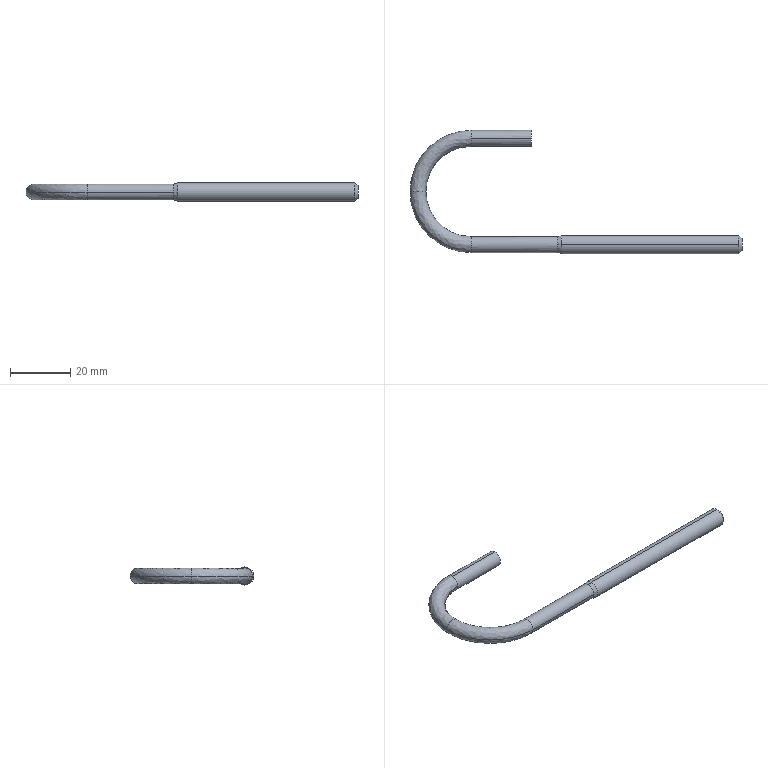Part | STEP file | 750038353 | 1 solid | 16 faces | box 110.3 x 40.95 x 6 mm | volume 4017 mm3 | spline 6 | cylinder 6 | cone 2 | plane 2 | commonest cylinder face diameters 5.3 x4 6 x2
STEP:
#1=CARTESIAN_POINT('',(28.594,-17.65,2.65));
#2=VERTEX_POINT('',#1);
#3=CARTESIAN_POINT('',(28.594,-15.,0.));
#4=VERTEX_POINT('',#3);
#5=CARTESIAN_POINT('',(28.594,-17.65,0.));
#6=DIRECTION('',(-1.,0.,0.));
#7=DIRECTION('',(0.,0.,-1.));
#8=AXIS2_PLACEMENT_3D('',#5,#6,#7);
#9=CIRCLE('',#8,2.65);
#10=EDGE_CURVE('',#2,#4,#9,.T.);
#11=ORIENTED_EDGE('',*,*,#10,.F.);
#12=CARTESIAN_POINT('',(30.,-17.65,3.));
#13=VERTEX_POINT('',#12);
#14=CARTESIAN_POINT('',(28.594,-17.65,5.65));
#15=DIRECTION('',(0.,-1.,0.));
#16=DIRECTION('',(0.,0.,1.));
#17=AXIS2_PLACEMENT_3D('',#14,#15,#16);
#18=CIRCLE('',#17,3.);
#19=EDGE_CURVE('',#2,#13,#18,.T.);
#20=ORIENTED_EDGE('',*,*,#19,.T.);
#21=CARTESIAN_POINT('',(30.,-17.65,-3.));
#22=VERTEX_POINT('',#21);
#23=CARTESIAN_POINT('',(30.,-17.65,0.));
#24=DIRECTION('',(1.,0.,0.));
#25=DIRECTION('',(0.,0.,-1.));
#26=AXIS2_PLACEMENT_3D('',#23,#24,#25);
#27=CIRCLE('',#26,3.);
#28=EDGE_CURVE('',#22,#13,#27,.T.);
#29=ORIENTED_EDGE('',*,*,#28,.F.);
#30=CARTESIAN_POINT('',(28.594,-17.65,-2.65));
#31=VERTEX_POINT('',#30);
#32=CARTESIAN_POINT('',(28.594,-17.65,-5.65));
#33=DIRECTION('',(0.,1.,0.));
#34=DIRECTION('',(0.,0.,-1.));
#35=AXIS2_PLACEMENT_3D('',#32,#33,#34);
#36=CIRCLE('',#35,3.);
#37=EDGE_CURVE('',#31,#22,#36,.T.);
#38=ORIENTED_EDGE('',*,*,#37,.F.);
#39=CARTESIAN_POINT('',(28.594,-17.65,0.));
#40=DIRECTION('',(-1.,0.,0.));
#41=DIRECTION('',(0.,0.,-1.));
#42=AXIS2_PLACEMENT_3D('',#39,#40,#41);
#43=CIRCLE('',#42,2.65);
#44=EDGE_CURVE('',#4,#31,#43,.T.);
#45=ORIENTED_EDGE('',*,*,#44,.F.);
#46=EDGE_LOOP('',(#11,#20,#29,#38,#45));
#47=FACE_OUTER_BOUND('',#46,.T.);
#48=CARTESIAN_POINT('',(28.594,-17.65,-2.65));
#49=CARTESIAN_POINT('',(28.594,-12.35,-2.65));
#50=CARTESIAN_POINT('',(28.594,-12.35,2.65));
#51=CARTESIAN_POINT('',(28.594,-17.65,2.65));
#52=CARTESIAN_POINT('',(29.087,-17.65,-2.65));
#53=CARTESIAN_POINT('',(29.087,-12.35,-2.65));
#54=CARTESIAN_POINT('',(29.087,-12.35,2.65));
#55=CARTESIAN_POINT('',(29.087,-17.65,2.65));
#56=CARTESIAN_POINT('',(29.565,-17.65,-2.769));
#57=CARTESIAN_POINT('',(29.565,-12.112,-2.769));
#58=CARTESIAN_POINT('',(29.565,-12.112,2.769));
#59=CARTESIAN_POINT('',(29.565,-17.65,2.769));
#60=CARTESIAN_POINT('',(30.,-17.65,-3.));
#61=CARTESIAN_POINT('',(30.,-11.65,-3.));
#62=CARTESIAN_POINT('',(30.,-11.65,3.));
#63=CARTESIAN_POINT('',(30.,-17.65,3.));
#64=(BOUNDED_SURFACE()B_SPLINE_SURFACE(3,3,((#48,#49,#50,#51),(#52,#53,#54,#55),(#56,#57,#58,#59),(#60,#61,#62,#63)),.UNSPECIFIED.,.F.,.F.,.F.)B_SPLINE_SURFACE_WITH_KNOTS((4,4),(4,4),(0.,1.),(0.,1.),.UNSPECIFIED.)GEOMETRIC_REPRESENTATION_ITEM()RATIONAL_B_SPLINE_SURFACE(((1.,0.3333,0.3333,1.),(0.9803,0.3268,0.3268,0.9803),(0.9803,0.3268,0.3268,0.9803),(1.,0.3333,0.3333,1.)))REPRESENTATION_ITEM('')SURFACE());
#65=ADVANCED_FACE('',(#47),#64,.F.);
#66=CARTESIAN_POINT('',(-15.,0.,0.));
#67=VERTEX_POINT('',#66);
#68=CARTESIAN_POINT('',(0.,15.,0.));
#69=VERTEX_POINT('',#68);
#70=CARTESIAN_POINT('',(0.,0.,0.));
#71=DIRECTION('',(0.,0.,-1.));
#72=DIRECTION('',(-1.,0.,0.));
#73=AXIS2_PLACEMENT_3D('',#70,#71,#72);
#74=CIRCLE('',#73,15.);
#75=EDGE_CURVE('',#67,#69,#74,.T.);
#76=ORIENTED_EDGE('',*,*,#75,.F.);
#77=CARTESIAN_POINT('',(-20.3,0.,0.));
#78=VERTEX_POINT('',#77);
#79=CARTESIAN_POINT('',(-17.65,0.,0.));
#80=DIRECTION('',(0.,1.,0.));
#81=DIRECTION('',(-1.,0.,0.));
#82=AXIS2_PLACEMENT_3D('',#79,#80,#81);
#83=CIRCLE('',#82,2.65);
#84=EDGE_CURVE('',#67,#78,#83,.T.);
#85=ORIENTED_EDGE('',*,*,#84,.T.);
#86=CARTESIAN_POINT('',(0.,20.3,0.));
#87=VERTEX_POINT('',#86);
#88=CARTESIAN_POINT('',(0.,0.,0.));
#89=DIRECTION('',(0.,0.,-1.));
#90=DIRECTION('',(-1.,0.,0.));
#91=AXIS2_PLACEMENT_3D('',#88,#89,#90);
#92=CIRCLE('',#91,20.3);
#93=EDGE_CURVE('',#78,#87,#92,.T.);
#94=ORIENTED_EDGE('',*,*,#93,.T.);
#95=CARTESIAN_POINT('',(0.,17.65,-2.65));
#96=VERTEX_POINT('',#95);
#97=CARTESIAN_POINT('',(0.,17.65,0.));
#98=DIRECTION('',(-1.,0.,0.));
#99=DIRECTION('',(0.,1.,0.));
#100=AXIS2_PLACEMENT_3D('',#97,#98,#99);
#101=CIRCLE('',#100,2.65);
#102=EDGE_CURVE('',#87,#96,#101,.T.);
#103=ORIENTED_EDGE('',*,*,#102,.T.);
#104=CARTESIAN_POINT('',(0.,17.65,0.));
#105=DIRECTION('',(-1.,0.,0.));
#106=DIRECTION('',(0.,1.,0.));
#107=AXIS2_PLACEMENT_3D('',#104,#105,#106);
#108=CIRCLE('',#107,2.65);
#109=EDGE_CURVE('',#96,#69,#108,.T.);
#110=ORIENTED_EDGE('',*,*,#109,.T.);
#111=EDGE_LOOP('',(#76,#85,#94,#103,#110));
#112=FACE_OUTER_BOUND('',#111,.T.);
#113=CARTESIAN_POINT('',(-15.,0.,0.));
#114=CARTESIAN_POINT('',(-15.,8.787,0.));
#115=CARTESIAN_POINT('',(-8.787,15.,0.));
#116=CARTESIAN_POINT('',(0.,15.,0.));
#117=CARTESIAN_POINT('',(-15.,0.,-5.3));
#118=CARTESIAN_POINT('',(-15.,8.787,-5.3));
#119=CARTESIAN_POINT('',(-8.787,15.,-5.3));
#120=CARTESIAN_POINT('',(0.,15.,-5.3));
#121=CARTESIAN_POINT('',(-20.3,0.,-5.3));
#122=CARTESIAN_POINT('',(-20.3,11.891,-5.3));
#123=CARTESIAN_POINT('',(-11.891,20.3,-5.3));
#124=CARTESIAN_POINT('',(0.,20.3,-5.3));
#125=CARTESIAN_POINT('',(-20.3,0.,0.));
#126=CARTESIAN_POINT('',(-20.3,11.891,0.));
#127=CARTESIAN_POINT('',(-11.891,20.3,0.));
#128=CARTESIAN_POINT('',(0.,20.3,0.));
#129=(BOUNDED_SURFACE()B_SPLINE_SURFACE(3,3,((#113,#114,#115,#116),(#117,#118,#119,#120),(#121,#122,#123,#124),(#125,#126,#127,#128)),.UNSPECIFIED.,.F.,.F.,.F.)B_SPLINE_SURFACE_WITH_KNOTS((4,4),(4,4),(0.,1.),(0.,1.),.UNSPECIFIED.)GEOMETRIC_REPRESENTATION_ITEM()RATIONAL_B_SPLINE_SURFACE(((1.,0.8047,0.8047,1.),(0.3333,0.2682,0.2682,0.3333),(0.3333,0.2682,0.2682,0.3333),(1.,0.8047,0.8047,1.)))REPRESENTATION_ITEM('')SURFACE());
#130=ADVANCED_FACE('',(#112),#129,.T.);
#131=ORIENTED_EDGE('',*,*,#93,.F.);
#132=CARTESIAN_POINT('',(-17.65,0.,0.));
#133=DIRECTION('',(0.,1.,0.));
#134=DIRECTION('',(-1.,0.,0.));
#135=AXIS2_PLACEMENT_3D('',#132,#133,#134);
#136=CIRCLE('',#135,2.65);
#137=EDGE_CURVE('',#78,#67,#136,.T.);
#138=ORIENTED_EDGE('',*,*,#137,.T.);
#139=ORIENTED_EDGE('',*,*,#75,.T.);
#140=CARTESIAN_POINT('',(0.,17.65,2.65));
#141=VERTEX_POINT('',#140);
#142=CARTESIAN_POINT('',(0.,17.65,0.));
#143=DIRECTION('',(-1.,0.,0.));
#144=DIRECTION('',(0.,1.,0.));
#145=AXIS2_PLACEMENT_3D('',#142,#143,#144);
#146=CIRCLE('',#145,2.65);
#147=EDGE_CURVE('',#69,#141,#146,.T.);
#148=ORIENTED_EDGE('',*,*,#147,.T.);
#149=CARTESIAN_POINT('',(0.,17.65,0.));
#150=DIRECTION('',(-1.,0.,0.));
#151=DIRECTION('',(0.,1.,0.));
#152=AXIS2_PLACEMENT_3D('',#149,#150,#151);
#153=CIRCLE('',#152,2.65);
#154=EDGE_CURVE('',#141,#87,#153,.T.);
#155=ORIENTED_EDGE('',*,*,#154,.T.);
#156=EDGE_LOOP('',(#131,#138,#139,#148,#155));
#157=FACE_OUTER_BOUND('',#156,.T.);
#158=CARTESIAN_POINT('',(-20.3,0.,0.));
#159=CARTESIAN_POINT('',(-20.3,11.891,0.));
#160=CARTESIAN_POINT('',(-11.891,20.3,0.));
#161=CARTESIAN_POINT('',(0.,20.3,0.));
#162=CARTESIAN_POINT('',(-20.3,0.,5.3));
#163=CARTESIAN_POINT('',(-20.3,11.891,5.3));
#164=CARTESIAN_POINT('',(-11.891,20.3,5.3));
#165=CARTESIAN_POINT('',(0.,20.3,5.3));
#166=CARTESIAN_POINT('',(-15.,0.,5.3));
#167=CARTESIAN_POINT('',(-15.,8.787,5.3));
#168=CARTESIAN_POINT('',(-8.787,15.,5.3));
#169=CARTESIAN_POINT('',(0.,15.,5.3));
#170=CARTESIAN_POINT('',(-15.,0.,0.));
#171=CARTESIAN_POINT('',(-15.,8.787,0.));
#172=CARTESIAN_POINT('',(-8.787,15.,0.));
#173=CARTESIAN_POINT('',(0.,15.,0.));
#174=(BOUNDED_SURFACE()B_SPLINE_SURFACE(3,3,((#158,#159,#160,#161),(#162,#163,#164,#165),(#166,#167,#168,#169),(#170,#171,#172,#173)),.UNSPECIFIED.,.F.,.F.,.F.)B_SPLINE_SURFACE_WITH_KNOTS((4,4),(4,4),(0.,1.),(0.,1.),.UNSPECIFIED.)GEOMETRIC_REPRESENTATION_ITEM()RATIONAL_B_SPLINE_SURFACE(((1.,0.8047,0.8047,1.),(0.3333,0.2682,0.2682,0.3333),(0.3333,0.2682,0.2682,0.3333),(1.,0.8047,0.8047,1.)))REPRESENTATION_ITEM('')SURFACE());
#175=ADVANCED_FACE('',(#157),#174,.T.);
#176=ORIENTED_EDGE('',*,*,#28,.T.);
#177=CARTESIAN_POINT('',(89.,-17.65,3.));
#178=VERTEX_POINT('',#177);
#179=CARTESIAN_POINT('',(30.,-17.65,3.));
#180=DIRECTION('',(1.,0.,0.));
#181=VECTOR('',#180,1000.);
#182=LINE('',#179,#181);
#183=EDGE_CURVE('',#13,#178,#182,.T.);
#184=ORIENTED_EDGE('',*,*,#183,.T.);
#185=CARTESIAN_POINT('',(89.,-17.65,-3.));
#186=VERTEX_POINT('',#185);
#187=CARTESIAN_POINT('',(89.,-17.65,0.));
#188=DIRECTION('',(-1.,0.,0.));
#189=DIRECTION('',(0.,0.,-1.));
#190=AXIS2_PLACEMENT_3D('',#187,#188,#189);
#191=CIRCLE('',#190,3.);
#192=EDGE_CURVE('',#178,#186,#191,.T.);
#193=ORIENTED_EDGE('',*,*,#192,.T.);
#194=CARTESIAN_POINT('',(30.,-17.65,-3.));
#195=DIRECTION('',(1.,0.,0.));
#196=VECTOR('',#195,1000.);
#197=LINE('',#194,#196);
#198=EDGE_CURVE('',#22,#186,#197,.T.);
#199=ORIENTED_EDGE('',*,*,#198,.F.);
#200=EDGE_LOOP('',(#176,#184,#193,#199));
#201=FACE_OUTER_BOUND('',#200,.T.);
#202=CARTESIAN_POINT('',(30.,-17.65,0.));
#203=DIRECTION('',(1.,0.,0.));
#204=DIRECTION('',(0.,0.,-1.));
#205=AXIS2_PLACEMENT_3D('',#202,#203,#204);
#206=CYLINDRICAL_SURFACE('',#205,3.);
#207=ADVANCED_FACE('',(#201),#206,.T.);
#208=CARTESIAN_POINT('',(90.,-17.65,2.));
#209=VERTEX_POINT('',#208);
#210=CARTESIAN_POINT('',(90.,-17.65,-2.));
#211=VERTEX_POINT('',#210);
#212=CARTESIAN_POINT('',(90.,-17.65,0.));
#213=DIRECTION('',(-1.,0.,0.));
#214=DIRECTION('',(0.,0.,1.));
#215=AXIS2_PLACEMENT_3D('',#212,#213,#214);
#216=CIRCLE('',#215,2.);
#217=EDGE_CURVE('',#209,#211,#216,.T.);
#218=ORIENTED_EDGE('',*,*,#217,.T.);
#219=CARTESIAN_POINT('',(89.,-17.65,-3.));
#220=DIRECTION('',(-0.7071,0.,-0.7071));
#221=VECTOR('',#220,1000.);
#222=LINE('',#219,#221);
#223=EDGE_CURVE('',#211,#186,#222,.T.);
#224=ORIENTED_EDGE('',*,*,#223,.T.);
#225=ORIENTED_EDGE('',*,*,#192,.F.);
#226=CARTESIAN_POINT('',(89.,-17.65,3.));
#227=DIRECTION('',(-0.7071,0.,0.7071));
#228=VECTOR('',#227,1000.);
#229=LINE('',#226,#228);
#230=EDGE_CURVE('',#209,#178,#229,.T.);
#231=ORIENTED_EDGE('',*,*,#230,.F.);
#232=EDGE_LOOP('',(#218,#224,#225,#231));
#233=FACE_OUTER_BOUND('',#232,.T.);
#234=CARTESIAN_POINT('',(89.,-17.65,0.));
#235=DIRECTION('',(-1.,0.,0.));
#236=DIRECTION('',(0.,0.,1.));
#237=AXIS2_PLACEMENT_3D('',#234,#235,#236);
#238=CONICAL_SURFACE('',#237,3.,0.7854);
#239=ADVANCED_FACE('',(#233),#238,.T.);
#240=CARTESIAN_POINT('',(0.,-15.,0.));
#241=VERTEX_POINT('',#240);
#242=CARTESIAN_POINT('',(0.,-20.3,0.));
#243=VERTEX_POINT('',#242);
#244=CARTESIAN_POINT('',(0.,-17.65,0.));
#245=DIRECTION('',(1.,0.,0.));
#246=DIRECTION('',(0.,1.,0.));
#247=AXIS2_PLACEMENT_3D('',#244,#245,#246);
#248=CIRCLE('',#247,2.65);
#249=EDGE_CURVE('',#241,#243,#248,.T.);
#250=ORIENTED_EDGE('',*,*,#249,.T.);
#251=CARTESIAN_POINT('',(28.594,-20.3,0.));
#252=VERTEX_POINT('',#251);
#253=CARTESIAN_POINT('',(0.,-20.3,0.));
#254=DIRECTION('',(1.,0.,0.));
#255=VECTOR('',#254,1000.);
#256=LINE('',#253,#255);
#257=EDGE_CURVE('',#243,#252,#256,.T.);
#258=ORIENTED_EDGE('',*,*,#257,.T.);
#259=CARTESIAN_POINT('',(28.594,-17.65,0.));
#260=DIRECTION('',(-1.,0.,0.));
#261=DIRECTION('',(0.,0.,-1.));
#262=AXIS2_PLACEMENT_3D('',#259,#260,#261);
#263=CIRCLE('',#262,2.65);
#264=EDGE_CURVE('',#252,#2,#263,.T.);
#265=ORIENTED_EDGE('',*,*,#264,.T.);
#266=ORIENTED_EDGE('',*,*,#10,.T.);
#267=CARTESIAN_POINT('',(0.,-15.,0.));
#268=DIRECTION('',(1.,0.,0.));
#269=VECTOR('',#268,1000.);
#270=LINE('',#267,#269);
#271=EDGE_CURVE('',#241,#4,#270,.T.);
#272=ORIENTED_EDGE('',*,*,#271,.F.);
#273=EDGE_LOOP('',(#250,#258,#265,#266,#272));
#274=FACE_OUTER_BOUND('',#273,.T.);
#275=CARTESIAN_POINT('',(0.,-17.65,0.));
#276=DIRECTION('',(1.,0.,0.));
#277=DIRECTION('',(0.,1.,0.));
#278=AXIS2_PLACEMENT_3D('',#275,#276,#277);
#279=CYLINDRICAL_SURFACE('',#278,2.65);
#280=ADVANCED_FACE('',(#274),#279,.T.);
#281=ORIENTED_EDGE('',*,*,#137,.F.);
#282=CARTESIAN_POINT('',(0.,0.,0.));
#283=DIRECTION('',(0.,0.,-1.));
#284=DIRECTION('',(-1.,0.,0.));
#285=AXIS2_PLACEMENT_3D('',#282,#283,#284);
#286=CIRCLE('',#285,20.3);
#287=EDGE_CURVE('',#243,#78,#286,.T.);
#288=ORIENTED_EDGE('',*,*,#287,.F.);
#289=ORIENTED_EDGE('',*,*,#249,.F.);
#290=CARTESIAN_POINT('',(0.,0.,0.));
#291=DIRECTION('',(0.,0.,-1.));
#292=DIRECTION('',(-1.,0.,0.));
#293=AXIS2_PLACEMENT_3D('',#290,#291,#292);
#294=CIRCLE('',#293,15.);
#295=EDGE_CURVE('',#241,#67,#294,.T.);
#296=ORIENTED_EDGE('',*,*,#295,.T.);
#297=EDGE_LOOP('',(#281,#288,#289,#296));
#298=FACE_OUTER_BOUND('',#297,.T.);
#299=CARTESIAN_POINT('',(0.,-20.3,0.));
#300=CARTESIAN_POINT('',(-11.891,-20.3,0.));
#301=CARTESIAN_POINT('',(-20.3,-11.891,0.));
#302=CARTESIAN_POINT('',(-20.3,0.,0.));
#303=CARTESIAN_POINT('',(0.,-20.3,5.3));
#304=CARTESIAN_POINT('',(-11.891,-20.3,5.3));
#305=CARTESIAN_POINT('',(-20.3,-11.891,5.3));
#306=CARTESIAN_POINT('',(-20.3,0.,5.3));
#307=CARTESIAN_POINT('',(0.,-15.,5.3));
#308=CARTESIAN_POINT('',(-8.787,-15.,5.3));
#309=CARTESIAN_POINT('',(-15.,-8.787,5.3));
#310=CARTESIAN_POINT('',(-15.,0.,5.3));
#311=CARTESIAN_POINT('',(0.,-15.,0.));
#312=CARTESIAN_POINT('',(-8.787,-15.,0.));
#313=CARTESIAN_POINT('',(-15.,-8.787,0.));
#314=CARTESIAN_POINT('',(-15.,0.,0.));
#315=(BOUNDED_SURFACE()B_SPLINE_SURFACE(3,3,((#299,#300,#301,#302),(#303,#304,#305,#306),(#307,#308,#309,#310),(#311,#312,#313,#314)),.UNSPECIFIED.,.F.,.F.,.T.)B_SPLINE_SURFACE_WITH_KNOTS((4,4),(4,4),(0.,1.),(0.,1.),.UNSPECIFIED.)GEOMETRIC_REPRESENTATION_ITEM()RATIONAL_B_SPLINE_SURFACE(((1.,0.8047,0.8047,1.),(0.3333,0.2682,0.2682,0.3333),(0.3333,0.2682,0.2682,0.3333),(1.,0.8047,0.8047,1.)))REPRESENTATION_ITEM('')SURFACE());
#316=ADVANCED_FACE('',(#298),#315,.T.);
#317=ORIENTED_EDGE('',*,*,#154,.F.);
#318=CARTESIAN_POINT('',(20.,17.65,2.65));
#319=VERTEX_POINT('',#318);
#320=CARTESIAN_POINT('',(0.,17.65,2.65));
#321=DIRECTION('',(1.,0.,0.));
#322=VECTOR('',#321,1000.);
#323=LINE('',#320,#322);
#324=EDGE_CURVE('',#141,#319,#323,.T.);
#325=ORIENTED_EDGE('',*,*,#324,.T.);
#326=CARTESIAN_POINT('',(20.,17.65,-2.65));
#327=VERTEX_POINT('',#326);
#328=CARTESIAN_POINT('',(20.,17.65,0.));
#329=DIRECTION('',(-1.,0.,0.));
#330=DIRECTION('',(0.,0.,-1.));
#331=AXIS2_PLACEMENT_3D('',#328,#329,#330);
#332=CIRCLE('',#331,2.65);
#333=EDGE_CURVE('',#319,#327,#332,.T.);
#334=ORIENTED_EDGE('',*,*,#333,.T.);
#335=CARTESIAN_POINT('',(0.,17.65,-2.65));
#336=DIRECTION('',(1.,0.,0.));
#337=VECTOR('',#336,1000.);
#338=LINE('',#335,#337);
#339=EDGE_CURVE('',#96,#327,#338,.T.);
#340=ORIENTED_EDGE('',*,*,#339,.F.);
#341=ORIENTED_EDGE('',*,*,#102,.F.);
#342=EDGE_LOOP('',(#317,#325,#334,#340,#341));
#343=FACE_OUTER_BOUND('',#342,.T.);
#344=CARTESIAN_POINT('',(0.,17.65,0.));
#345=DIRECTION('',(1.,0.,0.));
#346=DIRECTION('',(0.,0.,-1.));
#347=AXIS2_PLACEMENT_3D('',#344,#345,#346);
#348=CYLINDRICAL_SURFACE('',#347,2.65);
#349=ADVANCED_FACE('',(#343),#348,.T.);
#350=ORIENTED_EDGE('',*,*,#183,.F.);
#351=CARTESIAN_POINT('',(30.,-17.65,0.));
#352=DIRECTION('',(1.,0.,0.));
#353=DIRECTION('',(0.,0.,-1.));
#354=AXIS2_PLACEMENT_3D('',#351,#352,#353);
#355=CIRCLE('',#354,3.);
#356=EDGE_CURVE('',#13,#22,#355,.T.);
#357=ORIENTED_EDGE('',*,*,#356,.T.);
#358=ORIENTED_EDGE('',*,*,#198,.T.);
#359=CARTESIAN_POINT('',(89.,-17.65,0.));
#360=DIRECTION('',(-1.,0.,0.));
#361=DIRECTION('',(0.,0.,-1.));
#362=AXIS2_PLACEMENT_3D('',#359,#360,#361);
#363=CIRCLE('',#362,3.);
#364=EDGE_CURVE('',#186,#178,#363,.T.);
#365=ORIENTED_EDGE('',*,*,#364,.T.);
#366=EDGE_LOOP('',(#350,#357,#358,#365));
#367=FACE_OUTER_BOUND('',#366,.T.);
#368=CARTESIAN_POINT('',(30.,-17.65,0.));
#369=DIRECTION('',(1.,0.,0.));
#370=DIRECTION('',(0.,0.,-1.));
#371=AXIS2_PLACEMENT_3D('',#368,#369,#370);
#372=CYLINDRICAL_SURFACE('',#371,3.);
#373=ADVANCED_FACE('',(#367),#372,.T.);
#374=ORIENTED_EDGE('',*,*,#19,.F.);
#375=ORIENTED_EDGE('',*,*,#264,.F.);
#376=CARTESIAN_POINT('',(28.594,-17.65,0.));
#377=DIRECTION('',(-1.,0.,0.));
#378=DIRECTION('',(0.,0.,-1.));
#379=AXIS2_PLACEMENT_3D('',#376,#377,#378);
#380=CIRCLE('',#379,2.65);
#381=EDGE_CURVE('',#31,#252,#380,.T.);
#382=ORIENTED_EDGE('',*,*,#381,.F.);
#383=ORIENTED_EDGE('',*,*,#37,.T.);
#384=ORIENTED_EDGE('',*,*,#356,.F.);
#385=EDGE_LOOP('',(#374,#375,#382,#383,#384));
#386=FACE_OUTER_BOUND('',#385,.T.);
#387=CARTESIAN_POINT('',(28.594,-17.65,2.65));
#388=CARTESIAN_POINT('',(28.594,-22.95,2.65));
#389=CARTESIAN_POINT('',(28.594,-22.95,-2.65));
#390=CARTESIAN_POINT('',(28.594,-17.65,-2.65));
#391=CARTESIAN_POINT('',(29.087,-17.65,2.65));
#392=CARTESIAN_POINT('',(29.087,-22.95,2.65));
#393=CARTESIAN_POINT('',(29.087,-22.95,-2.65));
#394=CARTESIAN_POINT('',(29.087,-17.65,-2.65));
#395=CARTESIAN_POINT('',(29.565,-17.65,2.769));
#396=CARTESIAN_POINT('',(29.565,-23.188,2.769));
#397=CARTESIAN_POINT('',(29.565,-23.188,-2.769));
#398=CARTESIAN_POINT('',(29.565,-17.65,-2.769));
#399=CARTESIAN_POINT('',(30.,-17.65,3.));
#400=CARTESIAN_POINT('',(30.,-23.65,3.));
#401=CARTESIAN_POINT('',(30.,-23.65,-3.));
#402=CARTESIAN_POINT('',(30.,-17.65,-3.));
#403=(BOUNDED_SURFACE()B_SPLINE_SURFACE(3,3,((#387,#388,#389,#390),(#391,#392,#393,#394),(#395,#396,#397,#398),(#399,#400,#401,#402)),.UNSPECIFIED.,.F.,.F.,.F.)B_SPLINE_SURFACE_WITH_KNOTS((4,4),(4,4),(0.,1.),(0.,1.),.UNSPECIFIED.)GEOMETRIC_REPRESENTATION_ITEM()RATIONAL_B_SPLINE_SURFACE(((1.,0.3333,0.3333,1.),(0.9803,0.3268,0.3268,0.9803),(0.9803,0.3268,0.3268,0.9803),(1.,0.3333,0.3333,1.)))REPRESENTATION_ITEM('')SURFACE());
#404=ADVANCED_FACE('',(#386),#403,.F.);
#405=ORIENTED_EDGE('',*,*,#223,.F.);
#406=CARTESIAN_POINT('',(90.,-17.65,0.));
#407=DIRECTION('',(-1.,0.,0.));
#408=DIRECTION('',(0.,0.,1.));
#409=AXIS2_PLACEMENT_3D('',#406,#407,#408);
#410=CIRCLE('',#409,2.);
#411=EDGE_CURVE('',#211,#209,#410,.T.);
#412=ORIENTED_EDGE('',*,*,#411,.T.);
#413=ORIENTED_EDGE('',*,*,#230,.T.);
#414=ORIENTED_EDGE('',*,*,#364,.F.);
#415=EDGE_LOOP('',(#405,#412,#413,#414));
#416=FACE_OUTER_BOUND('',#415,.T.);
#417=CARTESIAN_POINT('',(89.,-17.65,0.));
#418=DIRECTION('',(-1.,0.,0.));
#419=DIRECTION('',(0.,0.,1.));
#420=AXIS2_PLACEMENT_3D('',#417,#418,#419);
#421=CONICAL_SURFACE('',#420,3.,0.7854);
#422=ADVANCED_FACE('',(#416),#421,.T.);
#423=ORIENTED_EDGE('',*,*,#257,.F.);
#424=CARTESIAN_POINT('',(0.,-17.65,0.));
#425=DIRECTION('',(1.,0.,0.));
#426=DIRECTION('',(0.,1.,0.));
#427=AXIS2_PLACEMENT_3D('',#424,#425,#426);
#428=CIRCLE('',#427,2.65);
#429=EDGE_CURVE('',#243,#241,#428,.T.);
#430=ORIENTED_EDGE('',*,*,#429,.T.);
#431=ORIENTED_EDGE('',*,*,#271,.T.);
#432=ORIENTED_EDGE('',*,*,#44,.T.);
#433=ORIENTED_EDGE('',*,*,#381,.T.);
#434=EDGE_LOOP('',(#423,#430,#431,#432,#433));
#435=FACE_OUTER_BOUND('',#434,.T.);
#436=CARTESIAN_POINT('',(0.,-17.65,0.));
#437=DIRECTION('',(1.,0.,0.));
#438=DIRECTION('',(0.,1.,0.));
#439=AXIS2_PLACEMENT_3D('',#436,#437,#438);
#440=CYLINDRICAL_SURFACE('',#439,2.65);
#441=ADVANCED_FACE('',(#435),#440,.T.);
#442=ORIENTED_EDGE('',*,*,#217,.F.);
#443=ORIENTED_EDGE('',*,*,#411,.F.);
#444=EDGE_LOOP('',(#442,#443));
#445=FACE_OUTER_BOUND('',#444,.T.);
#446=CARTESIAN_POINT('',(90.,-17.65,0.));
#447=DIRECTION('',(-1.,0.,0.));
#448=DIRECTION('',(0.,-1.,0.));
#449=AXIS2_PLACEMENT_3D('',#446,#447,#448);
#450=PLANE('',#449);
#451=ADVANCED_FACE('',(#445),#450,.F.);
#452=ORIENTED_EDGE('',*,*,#84,.F.);
#453=ORIENTED_EDGE('',*,*,#295,.F.);
#454=ORIENTED_EDGE('',*,*,#429,.F.);
#455=ORIENTED_EDGE('',*,*,#287,.T.);
#456=EDGE_LOOP('',(#452,#453,#454,#455));
#457=FACE_OUTER_BOUND('',#456,.T.);
#458=CARTESIAN_POINT('',(0.,-15.,0.));
#459=CARTESIAN_POINT('',(-8.787,-15.,0.));
#460=CARTESIAN_POINT('',(-15.,-8.787,0.));
#461=CARTESIAN_POINT('',(-15.,0.,0.));
#462=CARTESIAN_POINT('',(0.,-15.,-5.3));
#463=CARTESIAN_POINT('',(-8.787,-15.,-5.3));
#464=CARTESIAN_POINT('',(-15.,-8.787,-5.3));
#465=CARTESIAN_POINT('',(-15.,0.,-5.3));
#466=CARTESIAN_POINT('',(0.,-20.3,-5.3));
#467=CARTESIAN_POINT('',(-11.891,-20.3,-5.3));
#468=CARTESIAN_POINT('',(-20.3,-11.891,-5.3));
#469=CARTESIAN_POINT('',(-20.3,0.,-5.3));
#470=CARTESIAN_POINT('',(0.,-20.3,0.));
#471=CARTESIAN_POINT('',(-11.891,-20.3,0.));
#472=CARTESIAN_POINT('',(-20.3,-11.891,0.));
#473=CARTESIAN_POINT('',(-20.3,0.,0.));
#474=(BOUNDED_SURFACE()B_SPLINE_SURFACE(3,3,((#458,#459,#460,#461),(#462,#463,#464,#465),(#466,#467,#468,#469),(#470,#471,#472,#473)),.UNSPECIFIED.,.F.,.F.,.F.)B_SPLINE_SURFACE_WITH_KNOTS((4,4),(4,4),(0.,1.),(0.,1.),.UNSPECIFIED.)GEOMETRIC_REPRESENTATION_ITEM()RATIONAL_B_SPLINE_SURFACE(((1.,0.8047,0.8047,1.),(0.3333,0.2682,0.2682,0.3333),(0.3333,0.2682,0.2682,0.3333),(1.,0.8047,0.8047,1.)))REPRESENTATION_ITEM('')SURFACE());
#475=ADVANCED_FACE('',(#457),#474,.T.);
#476=ORIENTED_EDGE('',*,*,#324,.F.);
#477=ORIENTED_EDGE('',*,*,#147,.F.);
#478=ORIENTED_EDGE('',*,*,#109,.F.);
#479=ORIENTED_EDGE('',*,*,#339,.T.);
#480=CARTESIAN_POINT('',(20.,17.65,0.));
#481=DIRECTION('',(-1.,0.,0.));
#482=DIRECTION('',(0.,0.,-1.));
#483=AXIS2_PLACEMENT_3D('',#480,#481,#482);
#484=CIRCLE('',#483,2.65);
#485=EDGE_CURVE('',#327,#319,#484,.T.);
#486=ORIENTED_EDGE('',*,*,#485,.T.);
#487=EDGE_LOOP('',(#476,#477,#478,#479,#486));
#488=FACE_OUTER_BOUND('',#487,.T.);
#489=CARTESIAN_POINT('',(0.,17.65,0.));
#490=DIRECTION('',(1.,0.,0.));
#491=DIRECTION('',(0.,0.,-1.));
#492=AXIS2_PLACEMENT_3D('',#489,#490,#491);
#493=CYLINDRICAL_SURFACE('',#492,2.65);
#494=ADVANCED_FACE('',(#488),#493,.T.);
#495=ORIENTED_EDGE('',*,*,#485,.F.);
#496=ORIENTED_EDGE('',*,*,#333,.F.);
#497=EDGE_LOOP('',(#495,#496));
#498=FACE_OUTER_BOUND('',#497,.T.);
#499=CARTESIAN_POINT('',(20.,17.65,0.));
#500=DIRECTION('',(1.,0.,0.));
#501=DIRECTION('',(0.,1.,0.));
#502=AXIS2_PLACEMENT_3D('',#499,#500,#501);
#503=PLANE('',#502);
#504=ADVANCED_FACE('',(#498),#503,.T.);
#505=CLOSED_SHELL('',(#65,#130,#175,#207,#239,#280,#316,#349,#373,#404,#422,#441,#451,#475,#494,#504));
#506=MANIFOLD_SOLID_BREP('',#505);
#507=CARTESIAN_POINT('',(0.,0.,0.));
#508=DIRECTION('',(0.,0.,1.));
#509=DIRECTION('',(1.,0.,0.));
#510=AXIS2_PLACEMENT_3D('',#507,#508,#509);
#511=(LENGTH_UNIT()NAMED_UNIT(*)SI_UNIT(.MILLI.,.METRE.));
#512=UNCERTAINTY_MEASURE_WITH_UNIT(LENGTH_MEASURE(0.00001),#511,'','');
#513=(NAMED_UNIT(*)PLANE_ANGLE_UNIT()SI_UNIT($,.RADIAN.));
#514=(NAMED_UNIT(*)SI_UNIT($,.STERADIAN.)SOLID_ANGLE_UNIT());
#515=(GEOMETRIC_REPRESENTATION_CONTEXT(3)GLOBAL_UNCERTAINTY_ASSIGNED_CONTEXT((#512))GLOBAL_UNIT_ASSIGNED_CONTEXT((#511,#513,#514))REPRESENTATION_CONTEXT('',''));
#516=ADVANCED_BREP_SHAPE_REPRESENTATION('',(#506,#510),#515);